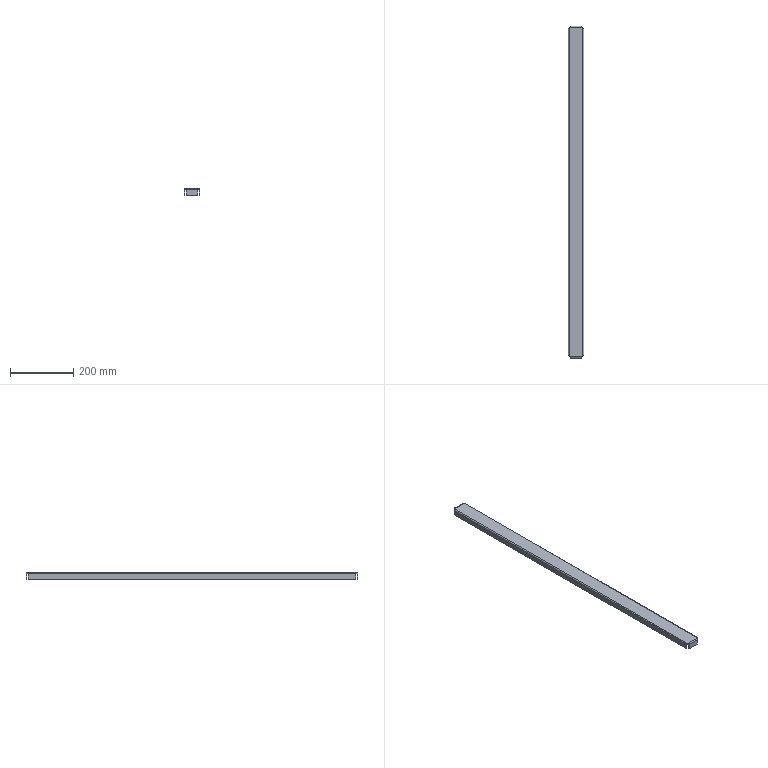Part | SolidWorks | features BaseBody 1 | 1 solid | 50 faces | box 50 x 1046 x 20 mm | volume 219402 mm3 | plane 42 | cylinder 8 | commonest cylinder face diameters 1.473 x4 6.473 x4
STEP:
#1=CARTESIAN_POINT('',(-18.,-520.5,-20.));
#2=VERTEX_POINT('',#1);
#3=CARTESIAN_POINT('',(18.,-520.5,-20.));
#4=VERTEX_POINT('',#3);
#5=CARTESIAN_POINT('',(18.,-520.5,-20.));
#6=DIRECTION('',(1.,0.,0.));
#7=VECTOR('',#6,1000.);
#8=LINE('',#5,#7);
#9=EDGE_CURVE('',#2,#4,#8,.T.);
#10=ORIENTED_EDGE('',*,*,#9,.T.);
#11=CARTESIAN_POINT('',(18.,-523.,-20.));
#12=VERTEX_POINT('',#11);
#13=CARTESIAN_POINT('',(18.,-523.,-20.));
#14=DIRECTION('',(0.,1.,0.));
#15=VECTOR('',#14,1000.);
#16=LINE('',#13,#15);
#17=EDGE_CURVE('',#12,#4,#16,.T.);
#18=ORIENTED_EDGE('',*,*,#17,.F.);
#19=CARTESIAN_POINT('',(-18.,-523.,-20.));
#20=VERTEX_POINT('',#19);
#21=CARTESIAN_POINT('',(0.,-523.,-20.));
#22=DIRECTION('',(1.,0.,0.));
#23=VECTOR('',#22,1000.);
#24=LINE('',#21,#23);
#25=EDGE_CURVE('',#20,#12,#24,.T.);
#26=ORIENTED_EDGE('',*,*,#25,.F.);
#27=CARTESIAN_POINT('',(-18.,-523.,-20.));
#28=DIRECTION('',(0.,1.,0.));
#29=VECTOR('',#28,1000.);
#30=LINE('',#27,#29);
#31=EDGE_CURVE('',#20,#2,#30,.T.);
#32=ORIENTED_EDGE('',*,*,#31,.T.);
#33=EDGE_LOOP('',(#10,#18,#26,#32));
#34=FACE_OUTER_BOUND('',#33,.T.);
#35=CARTESIAN_POINT('',(18.,-523.,-20.));
#36=DIRECTION('',(0.,0.,1.));
#37=DIRECTION('',(0.,-1.,0.));
#38=AXIS2_PLACEMENT_3D('',#35,#36,#37);
#39=PLANE('',#38);
#40=ADVANCED_FACE('',(#34),#39,.F.);
#41=CARTESIAN_POINT('',(-18.,-520.5,-3.237));
#42=VERTEX_POINT('',#41);
#43=CARTESIAN_POINT('',(-18.,-520.5,-20.));
#44=DIRECTION('',(0.,0.,-1.));
#45=VECTOR('',#44,1000.);
#46=LINE('',#43,#45);
#47=EDGE_CURVE('',#42,#2,#46,.T.);
#48=ORIENTED_EDGE('',*,*,#47,.F.);
#49=CARTESIAN_POINT('',(18.,-520.5,-3.237));
#50=VERTEX_POINT('',#49);
#51=CARTESIAN_POINT('',(18.,-520.5,-3.237));
#52=DIRECTION('',(-1.,0.,0.));
#53=VECTOR('',#52,1000.);
#54=LINE('',#51,#53);
#55=EDGE_CURVE('',#50,#42,#54,.T.);
#56=ORIENTED_EDGE('',*,*,#55,.F.);
#57=CARTESIAN_POINT('',(18.,-520.5,-2.5));
#58=DIRECTION('',(0.,0.,1.));
#59=VECTOR('',#58,1000.);
#60=LINE('',#57,#59);
#61=EDGE_CURVE('',#4,#50,#60,.T.);
#62=ORIENTED_EDGE('',*,*,#61,.F.);
#63=ORIENTED_EDGE('',*,*,#9,.F.);
#64=EDGE_LOOP('',(#48,#56,#62,#63));
#65=FACE_OUTER_BOUND('',#64,.T.);
#66=CARTESIAN_POINT('',(0.,-520.5,0.));
#67=DIRECTION('',(0.,1.,0.));
#68=DIRECTION('',(1.,0.,0.));
#69=AXIS2_PLACEMENT_3D('',#66,#67,#68);
#70=PLANE('',#69);
#71=ADVANCED_FACE('',(#65),#70,.T.);
#72=CARTESIAN_POINT('',(-18.,-523.,-3.237));
#73=VERTEX_POINT('',#72);
#74=CARTESIAN_POINT('',(18.,-523.,-3.237));
#75=VERTEX_POINT('',#74);
#76=CARTESIAN_POINT('',(18.,-523.,-3.237));
#77=DIRECTION('',(1.,0.,0.));
#78=VECTOR('',#77,1000.);
#79=LINE('',#76,#78);
#80=EDGE_CURVE('',#73,#75,#79,.T.);
#81=ORIENTED_EDGE('',*,*,#80,.F.);
#82=CARTESIAN_POINT('',(-18.,-523.,0.));
#83=DIRECTION('',(0.,0.,-1.));
#84=VECTOR('',#83,1000.);
#85=LINE('',#82,#84);
#86=EDGE_CURVE('',#73,#20,#85,.T.);
#87=ORIENTED_EDGE('',*,*,#86,.T.);
#88=ORIENTED_EDGE('',*,*,#25,.T.);
#89=CARTESIAN_POINT('',(18.,-523.,0.));
#90=DIRECTION('',(0.,0.,1.));
#91=VECTOR('',#90,1000.);
#92=LINE('',#89,#91);
#93=EDGE_CURVE('',#12,#75,#92,.T.);
#94=ORIENTED_EDGE('',*,*,#93,.T.);
#95=EDGE_LOOP('',(#81,#87,#88,#94));
#96=FACE_OUTER_BOUND('',#95,.T.);
#97=CARTESIAN_POINT('',(0.,-523.,0.));
#98=DIRECTION('',(0.,1.,0.));
#99=DIRECTION('',(1.,0.,0.));
#100=AXIS2_PLACEMENT_3D('',#97,#98,#99);
#101=PLANE('',#100);
#102=ADVANCED_FACE('',(#96),#101,.F.);
#103=CARTESIAN_POINT('',(18.,-523.,-3.237));
#104=DIRECTION('',(0.,-1.,0.));
#105=VECTOR('',#104,1000.);
#106=LINE('',#103,#105);
#107=EDGE_CURVE('',#50,#75,#106,.T.);
#108=ORIENTED_EDGE('',*,*,#107,.T.);
#109=ORIENTED_EDGE('',*,*,#93,.F.);
#110=ORIENTED_EDGE('',*,*,#17,.T.);
#111=ORIENTED_EDGE('',*,*,#61,.T.);
#112=EDGE_LOOP('',(#108,#109,#110,#111));
#113=FACE_OUTER_BOUND('',#112,.T.);
#114=CARTESIAN_POINT('',(18.,-523.,-2.5));
#115=DIRECTION('',(-1.,0.,0.));
#116=DIRECTION('',(0.,0.,1.));
#117=AXIS2_PLACEMENT_3D('',#114,#115,#116);
#118=PLANE('',#117);
#119=ADVANCED_FACE('',(#113),#118,.F.);
#120=CARTESIAN_POINT('',(-18.,-520.5,-3.237));
#121=DIRECTION('',(0.,-1.,0.));
#122=VECTOR('',#121,1000.);
#123=LINE('',#120,#122);
#124=EDGE_CURVE('',#42,#73,#123,.T.);
#125=ORIENTED_EDGE('',*,*,#124,.F.);
#126=ORIENTED_EDGE('',*,*,#47,.T.);
#127=ORIENTED_EDGE('',*,*,#31,.F.);
#128=ORIENTED_EDGE('',*,*,#86,.F.);
#129=EDGE_LOOP('',(#125,#126,#127,#128));
#130=FACE_OUTER_BOUND('',#129,.T.);
#131=CARTESIAN_POINT('',(-18.,-523.,-20.));
#132=DIRECTION('',(1.,0.,0.));
#133=DIRECTION('',(0.,-1.,0.));
#134=AXIS2_PLACEMENT_3D('',#131,#132,#133);
#135=PLANE('',#134);
#136=ADVANCED_FACE('',(#130),#135,.F.);
#137=CARTESIAN_POINT('',(-18.,-519.763,-2.5));
#138=VERTEX_POINT('',#137);
#139=CARTESIAN_POINT('',(18.,-519.763,-2.5));
#140=VERTEX_POINT('',#139);
#141=CARTESIAN_POINT('',(-18.,-519.763,-2.5));
#142=DIRECTION('',(1.,0.,0.));
#143=VECTOR('',#142,1000.);
#144=LINE('',#141,#143);
#145=EDGE_CURVE('',#138,#140,#144,.T.);
#146=ORIENTED_EDGE('',*,*,#145,.T.);
#147=CARTESIAN_POINT('',(18.,-519.763,-3.237));
#148=DIRECTION('',(1.,0.,0.));
#149=DIRECTION('',(0.,0.,1.));
#150=AXIS2_PLACEMENT_3D('',#147,#148,#149);
#151=CIRCLE('',#150,0.7366);
#152=EDGE_CURVE('',#140,#50,#151,.T.);
#153=ORIENTED_EDGE('',*,*,#152,.T.);
#154=ORIENTED_EDGE('',*,*,#55,.T.);
#155=CARTESIAN_POINT('',(-18.,-519.763,-3.237));
#156=DIRECTION('',(-1.,0.,0.));
#157=DIRECTION('',(0.,0.,1.));
#158=AXIS2_PLACEMENT_3D('',#155,#156,#157);
#159=CIRCLE('',#158,0.7366);
#160=EDGE_CURVE('',#42,#138,#159,.T.);
#161=ORIENTED_EDGE('',*,*,#160,.T.);
#162=EDGE_LOOP('',(#146,#153,#154,#161));
#163=FACE_OUTER_BOUND('',#162,.T.);
#164=CARTESIAN_POINT('',(-18.,-519.763,-3.237));
#165=DIRECTION('',(-1.,0.,0.));
#166=DIRECTION('',(0.,-1.,0.));
#167=AXIS2_PLACEMENT_3D('',#164,#165,#166);
#168=CYLINDRICAL_SURFACE('',#167,0.7366);
#169=ADVANCED_FACE('',(#163),#168,.F.);
#170=CARTESIAN_POINT('',(-18.,-519.763,0.));
#171=VERTEX_POINT('',#170);
#172=CARTESIAN_POINT('',(18.,-519.763,0.));
#173=VERTEX_POINT('',#172);
#174=CARTESIAN_POINT('',(-18.,-519.763,0.));
#175=DIRECTION('',(1.,0.,0.));
#176=VECTOR('',#175,1000.);
#177=LINE('',#174,#176);
#178=EDGE_CURVE('',#171,#173,#177,.T.);
#179=ORIENTED_EDGE('',*,*,#178,.F.);
#180=CARTESIAN_POINT('',(-18.,-522.915,-2.5));
#181=VERTEX_POINT('',#180);
#182=CARTESIAN_POINT('',(-18.,-519.763,-3.237));
#183=DIRECTION('',(-1.,0.,0.));
#184=DIRECTION('',(0.,0.,1.));
#185=AXIS2_PLACEMENT_3D('',#182,#183,#184);
#186=CIRCLE('',#185,3.237);
#187=EDGE_CURVE('',#181,#171,#186,.T.);
#188=ORIENTED_EDGE('',*,*,#187,.F.);
#189=CARTESIAN_POINT('',(-18.,-519.763,-3.237));
#190=DIRECTION('',(-1.,0.,0.));
#191=DIRECTION('',(0.,0.,1.));
#192=AXIS2_PLACEMENT_3D('',#189,#190,#191);
#193=CIRCLE('',#192,3.237);
#194=EDGE_CURVE('',#73,#181,#193,.T.);
#195=ORIENTED_EDGE('',*,*,#194,.F.);
#196=ORIENTED_EDGE('',*,*,#80,.T.);
#197=CARTESIAN_POINT('',(18.,-522.915,-2.5));
#198=VERTEX_POINT('',#197);
#199=CARTESIAN_POINT('',(18.,-519.763,-3.237));
#200=DIRECTION('',(1.,0.,0.));
#201=DIRECTION('',(0.,0.,1.));
#202=AXIS2_PLACEMENT_3D('',#199,#200,#201);
#203=CIRCLE('',#202,3.237);
#204=EDGE_CURVE('',#198,#75,#203,.T.);
#205=ORIENTED_EDGE('',*,*,#204,.F.);
#206=CARTESIAN_POINT('',(18.,-519.763,-3.237));
#207=DIRECTION('',(1.,0.,0.));
#208=DIRECTION('',(0.,0.,1.));
#209=AXIS2_PLACEMENT_3D('',#206,#207,#208);
#210=CIRCLE('',#209,3.237);
#211=EDGE_CURVE('',#173,#198,#210,.T.);
#212=ORIENTED_EDGE('',*,*,#211,.F.);
#213=EDGE_LOOP('',(#179,#188,#195,#196,#205,#212));
#214=FACE_OUTER_BOUND('',#213,.T.);
#215=CARTESIAN_POINT('',(-18.,-519.763,-3.237));
#216=DIRECTION('',(-1.,0.,0.));
#217=DIRECTION('',(0.,-1.,0.));
#218=AXIS2_PLACEMENT_3D('',#215,#216,#217);
#219=CYLINDRICAL_SURFACE('',#218,3.237);
#220=ADVANCED_FACE('',(#214),#219,.T.);
#221=ORIENTED_EDGE('',*,*,#194,.T.);
#222=CARTESIAN_POINT('',(-18.,-523.,-2.5));
#223=DIRECTION('',(0.,1.,0.));
#224=VECTOR('',#223,1000.);
#225=LINE('',#222,#224);
#226=EDGE_CURVE('',#181,#138,#225,.T.);
#227=ORIENTED_EDGE('',*,*,#226,.T.);
#228=ORIENTED_EDGE('',*,*,#160,.F.);
#229=ORIENTED_EDGE('',*,*,#124,.T.);
#230=EDGE_LOOP('',(#221,#227,#228,#229));
#231=FACE_OUTER_BOUND('',#230,.T.);
#232=CARTESIAN_POINT('',(-18.,-519.763,-3.237));
#233=DIRECTION('',(1.,0.,0.));
#234=DIRECTION('',(0.,1.,0.));
#235=AXIS2_PLACEMENT_3D('',#232,#233,#234);
#236=PLANE('',#235);
#237=ADVANCED_FACE('',(#231),#236,.F.);
#238=ORIENTED_EDGE('',*,*,#152,.F.);
#239=CARTESIAN_POINT('',(18.,-519.763,-2.5));
#240=DIRECTION('',(0.,-1.,0.));
#241=VECTOR('',#240,1000.);
#242=LINE('',#239,#241);
#243=EDGE_CURVE('',#140,#198,#242,.T.);
#244=ORIENTED_EDGE('',*,*,#243,.T.);
#245=ORIENTED_EDGE('',*,*,#204,.T.);
#246=ORIENTED_EDGE('',*,*,#107,.F.);
#247=EDGE_LOOP('',(#238,#244,#245,#246));
#248=FACE_OUTER_BOUND('',#247,.T.);
#249=CARTESIAN_POINT('',(18.,-519.763,-3.237));
#250=DIRECTION('',(1.,0.,0.));
#251=DIRECTION('',(0.,1.,0.));
#252=AXIS2_PLACEMENT_3D('',#249,#250,#251);
#253=PLANE('',#252);
#254=ADVANCED_FACE('',(#248),#253,.T.);
#255=CARTESIAN_POINT('',(22.5,-516.,-20.));
#256=VERTEX_POINT('',#255);
#257=CARTESIAN_POINT('',(22.5,516.,-20.));
#258=VERTEX_POINT('',#257);
#259=CARTESIAN_POINT('',(22.5,516.,-20.));
#260=DIRECTION('',(0.,1.,0.));
#261=VECTOR('',#260,1000.);
#262=LINE('',#259,#261);
#263=EDGE_CURVE('',#256,#258,#262,.T.);
#264=ORIENTED_EDGE('',*,*,#263,.T.);
#265=CARTESIAN_POINT('',(25.,516.,-20.));
#266=VERTEX_POINT('',#265);
#267=CARTESIAN_POINT('',(25.,516.,-20.));
#268=DIRECTION('',(-1.,0.,0.));
#269=VECTOR('',#268,1000.);
#270=LINE('',#267,#269);
#271=EDGE_CURVE('',#266,#258,#270,.T.);
#272=ORIENTED_EDGE('',*,*,#271,.F.);
#273=CARTESIAN_POINT('',(25.,-516.,-20.));
#274=VERTEX_POINT('',#273);
#275=CARTESIAN_POINT('',(25.,0.,-20.));
#276=DIRECTION('',(0.,1.,0.));
#277=VECTOR('',#276,1000.);
#278=LINE('',#275,#277);
#279=EDGE_CURVE('',#274,#266,#278,.T.);
#280=ORIENTED_EDGE('',*,*,#279,.F.);
#281=CARTESIAN_POINT('',(25.,-516.,-20.));
#282=DIRECTION('',(-1.,0.,0.));
#283=VECTOR('',#282,1000.);
#284=LINE('',#281,#283);
#285=EDGE_CURVE('',#274,#256,#284,.T.);
#286=ORIENTED_EDGE('',*,*,#285,.T.);
#287=EDGE_LOOP('',(#264,#272,#280,#286));
#288=FACE_OUTER_BOUND('',#287,.T.);
#289=CARTESIAN_POINT('',(25.,516.,-20.));
#290=DIRECTION('',(0.,0.,1.));
#291=DIRECTION('',(1.,0.,0.));
#292=AXIS2_PLACEMENT_3D('',#289,#290,#291);
#293=PLANE('',#292);
#294=ADVANCED_FACE('',(#288),#293,.F.);
#295=CARTESIAN_POINT('',(22.5,-516.,-3.237));
#296=VERTEX_POINT('',#295);
#297=CARTESIAN_POINT('',(22.5,-516.,-20.));
#298=DIRECTION('',(0.,0.,-1.));
#299=VECTOR('',#298,1000.);
#300=LINE('',#297,#299);
#301=EDGE_CURVE('',#296,#256,#300,.T.);
#302=ORIENTED_EDGE('',*,*,#301,.F.);
#303=CARTESIAN_POINT('',(22.5,516.,-3.237));
#304=VERTEX_POINT('',#303);
#305=CARTESIAN_POINT('',(22.5,516.,-3.237));
#306=DIRECTION('',(0.,-1.,0.));
#307=VECTOR('',#306,1000.);
#308=LINE('',#305,#307);
#309=EDGE_CURVE('',#304,#296,#308,.T.);
#310=ORIENTED_EDGE('',*,*,#309,.F.);
#311=CARTESIAN_POINT('',(22.5,516.,-2.5));
#312=DIRECTION('',(0.,0.,1.));
#313=VECTOR('',#312,1000.);
#314=LINE('',#311,#313);
#315=EDGE_CURVE('',#258,#304,#314,.T.);
#316=ORIENTED_EDGE('',*,*,#315,.F.);
#317=ORIENTED_EDGE('',*,*,#263,.F.);
#318=EDGE_LOOP('',(#302,#310,#316,#317));
#319=FACE_OUTER_BOUND('',#318,.T.);
#320=CARTESIAN_POINT('',(22.5,0.,0.));
#321=DIRECTION('',(-1.,0.,0.));
#322=DIRECTION('',(0.,0.,1.));
#323=AXIS2_PLACEMENT_3D('',#320,#321,#322);
#324=PLANE('',#323);
#325=ADVANCED_FACE('',(#319),#324,.T.);
#326=CARTESIAN_POINT('',(25.,-516.,-3.237));
#327=VERTEX_POINT('',#326);
#328=CARTESIAN_POINT('',(25.,516.,-3.237));
#329=VERTEX_POINT('',#328);
#330=CARTESIAN_POINT('',(25.,516.,-3.237));
#331=DIRECTION('',(0.,1.,0.));
#332=VECTOR('',#331,1000.);
#333=LINE('',#330,#332);
#334=EDGE_CURVE('',#327,#329,#333,.T.);
#335=ORIENTED_EDGE('',*,*,#334,.F.);
#336=CARTESIAN_POINT('',(25.,-516.,0.));
#337=DIRECTION('',(0.,0.,-1.));
#338=VECTOR('',#337,1000.);
#339=LINE('',#336,#338);
#340=EDGE_CURVE('',#327,#274,#339,.T.);
#341=ORIENTED_EDGE('',*,*,#340,.T.);
#342=ORIENTED_EDGE('',*,*,#279,.T.);
#343=CARTESIAN_POINT('',(25.,516.,0.));
#344=DIRECTION('',(0.,0.,1.));
#345=VECTOR('',#344,1000.);
#346=LINE('',#343,#345);
#347=EDGE_CURVE('',#266,#329,#346,.T.);
#348=ORIENTED_EDGE('',*,*,#347,.T.);
#349=EDGE_LOOP('',(#335,#341,#342,#348));
#350=FACE_OUTER_BOUND('',#349,.T.);
#351=CARTESIAN_POINT('',(25.,0.,0.));
#352=DIRECTION('',(-1.,0.,0.));
#353=DIRECTION('',(0.,0.,1.));
#354=AXIS2_PLACEMENT_3D('',#351,#352,#353);
#355=PLANE('',#354);
#356=ADVANCED_FACE('',(#350),#355,.F.);
#357=CARTESIAN_POINT('',(25.,516.,-3.237));
#358=DIRECTION('',(1.,0.,0.));
#359=VECTOR('',#358,1000.);
#360=LINE('',#357,#359);
#361=EDGE_CURVE('',#304,#329,#360,.T.);
#362=ORIENTED_EDGE('',*,*,#361,.T.);
#363=ORIENTED_EDGE('',*,*,#347,.F.);
#364=ORIENTED_EDGE('',*,*,#271,.T.);
#365=ORIENTED_EDGE('',*,*,#315,.T.);
#366=EDGE_LOOP('',(#362,#363,#364,#365));
#367=FACE_OUTER_BOUND('',#366,.T.);
#368=CARTESIAN_POINT('',(25.,516.,-2.5));
#369=DIRECTION('',(0.,-1.,0.));
#370=DIRECTION('',(-1.,0.,0.));
#371=AXIS2_PLACEMENT_3D('',#368,#369,#370);
#372=PLANE('',#371);
#373=ADVANCED_FACE('',(#367),#372,.F.);
#374=CARTESIAN_POINT('',(22.5,-516.,-3.237));
#375=DIRECTION('',(1.,0.,0.));
#376=VECTOR('',#375,1000.);
#377=LINE('',#374,#376);
#378=EDGE_CURVE('',#296,#327,#377,.T.);
#379=ORIENTED_EDGE('',*,*,#378,.F.);
#380=ORIENTED_EDGE('',*,*,#301,.T.);
#381=ORIENTED_EDGE('',*,*,#285,.F.);
#382=ORIENTED_EDGE('',*,*,#340,.F.);
#383=EDGE_LOOP('',(#379,#380,#381,#382));
#384=FACE_OUTER_BOUND('',#383,.T.);
#385=CARTESIAN_POINT('',(25.,-516.,-20.));
#386=DIRECTION('',(0.,1.,0.));
#387=DIRECTION('',(0.,0.,-1.));
#388=AXIS2_PLACEMENT_3D('',#385,#386,#387);
#389=PLANE('',#388);
#390=ADVANCED_FACE('',(#384),#389,.F.);
#391=CARTESIAN_POINT('',(21.763,-516.,-2.5));
#392=VERTEX_POINT('',#391);
#393=CARTESIAN_POINT('',(21.763,516.,-2.5));
#394=VERTEX_POINT('',#393);
#395=CARTESIAN_POINT('',(21.763,-516.,-2.5));
#396=DIRECTION('',(0.,1.,0.));
#397=VECTOR('',#396,1000.);
#398=LINE('',#395,#397);
#399=EDGE_CURVE('',#392,#394,#398,.T.);
#400=ORIENTED_EDGE('',*,*,#399,.T.);
#401=CARTESIAN_POINT('',(21.763,516.,-3.237));
#402=DIRECTION('',(0.,1.,0.));
#403=DIRECTION('',(0.,0.,-1.));
#404=AXIS2_PLACEMENT_3D('',#401,#402,#403);
#405=CIRCLE('',#404,0.7366);
#406=EDGE_CURVE('',#394,#304,#405,.T.);
#407=ORIENTED_EDGE('',*,*,#406,.T.);
#408=ORIENTED_EDGE('',*,*,#309,.T.);
#409=CARTESIAN_POINT('',(21.763,-516.,-3.237));
#410=DIRECTION('',(0.,-1.,0.));
#411=DIRECTION('',(0.,0.,-1.));
#412=AXIS2_PLACEMENT_3D('',#409,#410,#411);
#413=CIRCLE('',#412,0.7366);
#414=EDGE_CURVE('',#296,#392,#413,.T.);
#415=ORIENTED_EDGE('',*,*,#414,.T.);
#416=EDGE_LOOP('',(#400,#407,#408,#415));
#417=FACE_OUTER_BOUND('',#416,.T.);
#418=CARTESIAN_POINT('',(21.763,-516.,-3.237));
#419=DIRECTION('',(0.,-1.,0.));
#420=DIRECTION('',(1.,0.,0.));
#421=AXIS2_PLACEMENT_3D('',#418,#419,#420);
#422=CYLINDRICAL_SURFACE('',#421,0.7366);
#423=ADVANCED_FACE('',(#417),#422,.F.);
#424=CARTESIAN_POINT('',(21.763,-516.,0.));
#425=VERTEX_POINT('',#424);
#426=CARTESIAN_POINT('',(21.763,516.,0.));
#427=VERTEX_POINT('',#426);
#428=CARTESIAN_POINT('',(21.763,-516.,0.));
#429=DIRECTION('',(0.,1.,0.));
#430=VECTOR('',#429,1000.);
#431=LINE('',#428,#430);
#432=EDGE_CURVE('',#425,#427,#431,.T.);
#433=ORIENTED_EDGE('',*,*,#432,.F.);
#434=CARTESIAN_POINT('',(24.915,-516.,-2.5));
#435=VERTEX_POINT('',#434);
#436=CARTESIAN_POINT('',(21.763,-516.,-3.237));
#437=DIRECTION('',(0.,-1.,0.));
#438=DIRECTION('',(0.,0.,-1.));
#439=AXIS2_PLACEMENT_3D('',#436,#437,#438);
#440=CIRCLE('',#439,3.237);
#441=EDGE_CURVE('',#435,#425,#440,.T.);
#442=ORIENTED_EDGE('',*,*,#441,.F.);
#443=CARTESIAN_POINT('',(21.763,-516.,-3.237));
#444=DIRECTION('',(0.,-1.,0.));
#445=DIRECTION('',(0.,0.,-1.));
#446=AXIS2_PLACEMENT_3D('',#443,#444,#445);
#447=CIRCLE('',#446,3.237);
#448=EDGE_CURVE('',#327,#435,#447,.T.);
#449=ORIENTED_EDGE('',*,*,#448,.F.);
#450=ORIENTED_EDGE('',*,*,#334,.T.);
#451=CARTESIAN_POINT('',(24.915,516.,-2.5));
#452=VERTEX_POINT('',#451);
#453=CARTESIAN_POINT('',(21.763,516.,-3.237));
#454=DIRECTION('',(0.,1.,0.));
#455=DIRECTION('',(0.,0.,-1.));
#456=AXIS2_PLACEMENT_3D('',#453,#454,#455);
#457=CIRCLE('',#456,3.237);
#458=EDGE_CURVE('',#452,#329,#457,.T.);
#459=ORIENTED_EDGE('',*,*,#458,.F.);
#460=CARTESIAN_POINT('',(21.763,516.,-3.237));
#461=DIRECTION('',(0.,1.,0.));
#462=DIRECTION('',(0.,0.,-1.));
#463=AXIS2_PLACEMENT_3D('',#460,#461,#462);
#464=CIRCLE('',#463,3.237);
#465=EDGE_CURVE('',#427,#452,#464,.T.);
#466=ORIENTED_EDGE('',*,*,#465,.F.);
#467=EDGE_LOOP('',(#433,#442,#449,#450,#459,#466));
#468=FACE_OUTER_BOUND('',#467,.T.);
#469=CARTESIAN_POINT('',(21.763,-516.,-3.237));
#470=DIRECTION('',(0.,-1.,0.));
#471=DIRECTION('',(1.,0.,0.));
#472=AXIS2_PLACEMENT_3D('',#469,#470,#471);
#473=CYLINDRICAL_SURFACE('',#472,3.237);
#474=ADVANCED_FACE('',(#468),#473,.T.);
#475=ORIENTED_EDGE('',*,*,#448,.T.);
#476=CARTESIAN_POINT('',(25.,-516.,-2.5));
#477=DIRECTION('',(-1.,0.,0.));
#478=VECTOR('',#477,1000.);
#479=LINE('',#476,#478);
#480=EDGE_CURVE('',#435,#392,#479,.T.);
#481=ORIENTED_EDGE('',*,*,#480,.T.);
#482=ORIENTED_EDGE('',*,*,#414,.F.);
#483=ORIENTED_EDGE('',*,*,#378,.T.);
#484=EDGE_LOOP('',(#475,#481,#482,#483));
#485=FACE_OUTER_BOUND('',#484,.T.);
#486=CARTESIAN_POINT('',(21.763,-516.,-3.237));
#487=DIRECTION('',(0.,1.,0.));
#488=DIRECTION('',(1.,0.,0.));
#489=AXIS2_PLACEMENT_3D('',#486,#487,#488);
#490=PLANE('',#489);
#491=ADVANCED_FACE('',(#485),#490,.F.);
#492=ORIENTED_EDGE('',*,*,#406,.F.);
#493=CARTESIAN_POINT('',(21.763,516.,-2.5));
#494=DIRECTION('',(1.,0.,0.));
#495=VECTOR('',#494,1000.);
#496=LINE('',#493,#495);
#497=EDGE_CURVE('',#394,#452,#496,.T.);
#498=ORIENTED_EDGE('',*,*,#497,.T.);
#499=ORIENTED_EDGE('',*,*,#458,.T.);
#500=ORIENTED_EDGE('',*,*,#361,.F.);
#501=EDGE_LOOP('',(#492,#498,#499,#500));
#502=FACE_OUTER_BOUND('',#501,.T.);
#503=CARTESIAN_POINT('',(21.763,516.,-3.237));
#504=DIRECTION('',(0.,1.,0.));
#505=DIRECTION('',(1.,0.,0.));
#506=AXIS2_PLACEMENT_3D('',#503,#504,#505);
#507=PLANE('',#506);
#508=ADVANCED_FACE('',(#502),#507,.T.);
#509=CARTESIAN_POINT('',(18.,520.5,-20.));
#510=VERTEX_POINT('',#509);
#511=CARTESIAN_POINT('',(-18.,520.5,-20.));
#512=VERTEX_POINT('',#511);
#513=CARTESIAN_POINT('',(-18.,520.5,-20.));
#514=DIRECTION('',(-1.,0.,0.));
#515=VECTOR('',#514,1000.);
#516=LINE('',#513,#515);
#517=EDGE_CURVE('',#510,#512,#516,.T.);
#518=ORIENTED_EDGE('',*,*,#517,.T.);
#519=CARTESIAN_POINT('',(-18.,523.,-20.));
#520=VERTEX_POINT('',#519);
#521=CARTESIAN_POINT('',(-18.,523.,-20.));
#522=DIRECTION('',(0.,-1.,0.));
#523=VECTOR('',#522,1000.);
#524=LINE('',#521,#523);
#525=EDGE_CURVE('',#520,#512,#524,.T.);
#526=ORIENTED_EDGE('',*,*,#525,.F.);
#527=CARTESIAN_POINT('',(18.,523.,-20.));
#528=VERTEX_POINT('',#527);
#529=CARTESIAN_POINT('',(0.,523.,-20.));
#530=DIRECTION('',(-1.,0.,0.));
#531=VECTOR('',#530,1000.);
#532=LINE('',#529,#531);
#533=EDGE_CURVE('',#528,#520,#532,.T.);
#534=ORIENTED_EDGE('',*,*,#533,.F.);
#535=CARTESIAN_POINT('',(18.,523.,-20.));
#536=DIRECTION('',(0.,-1.,0.));
#537=VECTOR('',#536,1000.);
#538=LINE('',#535,#537);
#539=EDGE_CURVE('',#528,#510,#538,.T.);
#540=ORIENTED_EDGE('',*,*,#539,.T.);
#541=EDGE_LOOP('',(#518,#526,#534,#540));
#542=FACE_OUTER_BOUND('',#541,.T.);
#543=CARTESIAN_POINT('',(-18.,523.,-20.));
#544=DIRECTION('',(0.,0.,1.));
#545=DIRECTION('',(0.,-1.,0.));
#546=AXIS2_PLACEMENT_3D('',#543,#544,#545);
#547=PLANE('',#546);
#548=ADVANCED_FACE('',(#542),#547,.F.);
#549=CARTESIAN_POINT('',(18.,520.5,-3.237));
#550=VERTEX_POINT('',#549);
#551=CARTESIAN_POINT('',(18.,520.5,-20.));
#552=DIRECTION('',(0.,0.,-1.));
#553=VECTOR('',#552,1000.);
#554=LINE('',#551,#553);
#555=EDGE_CURVE('',#550,#510,#554,.T.);
#556=ORIENTED_EDGE('',*,*,#555,.F.);
#557=CARTESIAN_POINT('',(-18.,520.5,-3.237));
#558=VERTEX_POINT('',#557);
#559=CARTESIAN_POINT('',(-18.,520.5,-3.237));
#560=DIRECTION('',(1.,0.,0.));
#561=VECTOR('',#560,1000.);
#562=LINE('',#559,#561);
#563=EDGE_CURVE('',#558,#550,#562,.T.);
#564=ORIENTED_EDGE('',*,*,#563,.F.);
#565=CARTESIAN_POINT('',(-18.,520.5,-2.5));
#566=DIRECTION('',(0.,0.,1.));
#567=VECTOR('',#566,1000.);
#568=LINE('',#565,#567);
#569=EDGE_CURVE('',#512,#558,#568,.T.);
#570=ORIENTED_EDGE('',*,*,#569,.F.);
#571=ORIENTED_EDGE('',*,*,#517,.F.);
#572=EDGE_LOOP('',(#556,#564,#570,#571));
#573=FACE_OUTER_BOUND('',#572,.T.);
#574=CARTESIAN_POINT('',(0.,520.5,0.));
#575=DIRECTION('',(0.,-1.,0.));
#576=DIRECTION('',(0.,0.,-1.));
#577=AXIS2_PLACEMENT_3D('',#574,#575,#576);
#578=PLANE('',#577);
#579=ADVANCED_FACE('',(#573),#578,.T.);
#580=CARTESIAN_POINT('',(18.,523.,-3.237));
#581=VERTEX_POINT('',#580);
#582=CARTESIAN_POINT('',(-18.,523.,-3.237));
#583=VERTEX_POINT('',#582);
#584=CARTESIAN_POINT('',(-18.,523.,-3.237));
#585=DIRECTION('',(-1.,0.,0.));
#586=VECTOR('',#585,1000.);
#587=LINE('',#584,#586);
#588=EDGE_CURVE('',#581,#583,#587,.T.);
#589=ORIENTED_EDGE('',*,*,#588,.F.);
#590=CARTESIAN_POINT('',(18.,523.,0.));
#591=DIRECTION('',(0.,0.,-1.));
#592=VECTOR('',#591,1000.);
#593=LINE('',#590,#592);
#594=EDGE_CURVE('',#581,#528,#593,.T.);
#595=ORIENTED_EDGE('',*,*,#594,.T.);
#596=ORIENTED_EDGE('',*,*,#533,.T.);
#597=CARTESIAN_POINT('',(-18.,523.,0.));
#598=DIRECTION('',(0.,0.,1.));
#599=VECTOR('',#598,1000.);
#600=LINE('',#597,#599);
#601=EDGE_CURVE('',#520,#583,#600,.T.);
#602=ORIENTED_EDGE('',*,*,#601,.T.);
#603=EDGE_LOOP('',(#589,#595,#596,#602));
#604=FACE_OUTER_BOUND('',#603,.T.);
#605=CARTESIAN_POINT('',(0.,523.,0.));
#606=DIRECTION('',(0.,-1.,0.));
#607=DIRECTION('',(0.,0.,-1.));
#608=AXIS2_PLACEMENT_3D('',#605,#606,#607);
#609=PLANE('',#608);
#610=ADVANCED_FACE('',(#604),#609,.F.);
#611=CARTESIAN_POINT('',(-18.,523.,-3.237));
#612=DIRECTION('',(0.,1.,0.));
#613=VECTOR('',#612,1000.);
#614=LINE('',#611,#613);
#615=EDGE_CURVE('',#558,#583,#614,.T.);
#616=ORIENTED_EDGE('',*,*,#615,.T.);
#617=ORIENTED_EDGE('',*,*,#601,.F.);
#618=ORIENTED_EDGE('',*,*,#525,.T.);
#619=ORIENTED_EDGE('',*,*,#569,.T.);
#620=EDGE_LOOP('',(#616,#617,#618,#619));
#621=FACE_OUTER_BOUND('',#620,.T.);
#622=CARTESIAN_POINT('',(-18.,523.,-2.5));
#623=DIRECTION('',(1.,0.,0.));
#624=DIRECTION('',(0.,1.,0.));
#625=AXIS2_PLACEMENT_3D('',#622,#623,#624);
#626=PLANE('',#625);
#627=ADVANCED_FACE('',(#621),#626,.F.);
#628=CARTESIAN_POINT('',(18.,520.5,-3.237));
#629=DIRECTION('',(0.,1.,0.));
#630=VECTOR('',#629,1000.);
#631=LINE('',#628,#630);
#632=EDGE_CURVE('',#550,#581,#631,.T.);
#633=ORIENTED_EDGE('',*,*,#632,.F.);
#634=ORIENTED_EDGE('',*,*,#555,.T.);
#635=ORIENTED_EDGE('',*,*,#539,.F.);
#636=ORIENTED_EDGE('',*,*,#594,.F.);
#637=EDGE_LOOP('',(#633,#634,#635,#636));
#638=FACE_OUTER_BOUND('',#637,.T.);
#639=CARTESIAN_POINT('',(18.,523.,-20.));
#640=DIRECTION('',(-1.,0.,0.));
#641=DIRECTION('',(0.,1.,0.));
#642=AXIS2_PLACEMENT_3D('',#639,#640,#641);
#643=PLANE('',#642);
#644=ADVANCED_FACE('',(#638),#643,.F.);
#645=CARTESIAN_POINT('',(18.,519.763,-2.5));
#646=VERTEX_POINT('',#645);
#647=CARTESIAN_POINT('',(-18.,519.763,-2.5));
#648=VERTEX_POINT('',#647);
#649=CARTESIAN_POINT('',(18.,519.763,-2.5));
#650=DIRECTION('',(-1.,0.,0.));
#651=VECTOR('',#650,1000.);
#652=LINE('',#649,#651);
#653=EDGE_CURVE('',#646,#648,#652,.T.);
#654=ORIENTED_EDGE('',*,*,#653,.T.);
#655=CARTESIAN_POINT('',(-18.,519.763,-3.237));
#656=DIRECTION('',(-1.,0.,0.));
#657=DIRECTION('',(0.,0.,-1.));
#658=AXIS2_PLACEMENT_3D('',#655,#656,#657);
#659=CIRCLE('',#658,0.7366);
#660=EDGE_CURVE('',#648,#558,#659,.T.);
#661=ORIENTED_EDGE('',*,*,#660,.T.);
#662=ORIENTED_EDGE('',*,*,#563,.T.);
#663=CARTESIAN_POINT('',(18.,519.763,-3.237));
#664=DIRECTION('',(1.,0.,0.));
#665=DIRECTION('',(0.,0.,-1.));
#666=AXIS2_PLACEMENT_3D('',#663,#664,#665);
#667=CIRCLE('',#666,0.7366);
#668=EDGE_CURVE('',#550,#646,#667,.T.);
#669=ORIENTED_EDGE('',*,*,#668,.T.);
#670=EDGE_LOOP('',(#654,#661,#662,#669));
#671=FACE_OUTER_BOUND('',#670,.T.);
#672=CARTESIAN_POINT('',(18.,519.763,-3.237));
#673=DIRECTION('',(1.,0.,0.));
#674=DIRECTION('',(0.,1.,0.));
#675=AXIS2_PLACEMENT_3D('',#672,#673,#674);
#676=CYLINDRICAL_SURFACE('',#675,0.7366);
#677=ADVANCED_FACE('',(#671),#676,.F.);
#678=CARTESIAN_POINT('',(18.,519.763,0.));
#679=VERTEX_POINT('',#678);
#680=CARTESIAN_POINT('',(-18.,519.763,0.));
#681=VERTEX_POINT('',#680);
#682=CARTESIAN_POINT('',(18.,519.763,0.));
#683=DIRECTION('',(-1.,0.,0.));
#684=VECTOR('',#683,1000.);
#685=LINE('',#682,#684);
#686=EDGE_CURVE('',#679,#681,#685,.T.);
#687=ORIENTED_EDGE('',*,*,#686,.F.);
#688=CARTESIAN_POINT('',(18.,522.915,-2.5));
#689=VERTEX_POINT('',#688);
#690=CARTESIAN_POINT('',(18.,519.763,-3.237));
#691=DIRECTION('',(1.,0.,0.));
#692=DIRECTION('',(0.,0.,-1.));
#693=AXIS2_PLACEMENT_3D('',#690,#691,#692);
#694=CIRCLE('',#693,3.237);
#695=EDGE_CURVE('',#689,#679,#694,.T.);
#696=ORIENTED_EDGE('',*,*,#695,.F.);
#697=CARTESIAN_POINT('',(18.,519.763,-3.237));
#698=DIRECTION('',(1.,0.,0.));
#699=DIRECTION('',(0.,0.,-1.));
#700=AXIS2_PLACEMENT_3D('',#697,#698,#699);
#701=CIRCLE('',#700,3.237);
#702=EDGE_CURVE('',#581,#689,#701,.T.);
#703=ORIENTED_EDGE('',*,*,#702,.F.);
#704=ORIENTED_EDGE('',*,*,#588,.T.);
#705=CARTESIAN_POINT('',(-18.,522.915,-2.5));
#706=VERTEX_POINT('',#705);
#707=CARTESIAN_POINT('',(-18.,519.763,-3.237));
#708=DIRECTION('',(-1.,0.,0.));
#709=DIRECTION('',(0.,0.,-1.));
#710=AXIS2_PLACEMENT_3D('',#707,#708,#709);
#711=CIRCLE('',#710,3.237);
#712=EDGE_CURVE('',#706,#583,#711,.T.);
#713=ORIENTED_EDGE('',*,*,#712,.F.);
#714=CARTESIAN_POINT('',(-18.,519.763,-3.237));
#715=DIRECTION('',(-1.,0.,0.));
#716=DIRECTION('',(0.,0.,-1.));
#717=AXIS2_PLACEMENT_3D('',#714,#715,#716);
#718=CIRCLE('',#717,3.237);
#719=EDGE_CURVE('',#681,#706,#718,.T.);
#720=ORIENTED_EDGE('',*,*,#719,.F.);
#721=EDGE_LOOP('',(#687,#696,#703,#704,#713,#720));
#722=FACE_OUTER_BOUND('',#721,.T.);
#723=CARTESIAN_POINT('',(18.,519.763,-3.237));
#724=DIRECTION('',(1.,0.,0.));
#725=DIRECTION('',(0.,1.,0.));
#726=AXIS2_PLACEMENT_3D('',#723,#724,#725);
#727=CYLINDRICAL_SURFACE('',#726,3.237);
#728=ADVANCED_FACE('',(#722),#727,.T.);
#729=ORIENTED_EDGE('',*,*,#702,.T.);
#730=CARTESIAN_POINT('',(18.,523.,-2.5));
#731=DIRECTION('',(0.,-1.,0.));
#732=VECTOR('',#731,1000.);
#733=LINE('',#730,#732);
#734=EDGE_CURVE('',#689,#646,#733,.T.);
#735=ORIENTED_EDGE('',*,*,#734,.T.);
#736=ORIENTED_EDGE('',*,*,#668,.F.);
#737=ORIENTED_EDGE('',*,*,#632,.T.);
#738=EDGE_LOOP('',(#729,#735,#736,#737));
#739=FACE_OUTER_BOUND('',#738,.T.);
#740=CARTESIAN_POINT('',(18.,519.763,-3.237));
#741=DIRECTION('',(-1.,0.,0.));
#742=DIRECTION('',(0.,0.,1.));
#743=AXIS2_PLACEMENT_3D('',#740,#741,#742);
#744=PLANE('',#743);
#745=ADVANCED_FACE('',(#739),#744,.F.);
#746=ORIENTED_EDGE('',*,*,#660,.F.);
#747=CARTESIAN_POINT('',(-18.,519.763,-2.5));
#748=DIRECTION('',(0.,1.,0.));
#749=VECTOR('',#748,1000.);
#750=LINE('',#747,#749);
#751=EDGE_CURVE('',#648,#706,#750,.T.);
#752=ORIENTED_EDGE('',*,*,#751,.T.);
#753=ORIENTED_EDGE('',*,*,#712,.T.);
#754=ORIENTED_EDGE('',*,*,#615,.F.);
#755=EDGE_LOOP('',(#746,#752,#753,#754));
#756=FACE_OUTER_BOUND('',#755,.T.);
#757=CARTESIAN_POINT('',(-18.,519.763,-3.237));
#758=DIRECTION('',(-1.,0.,0.));
#759=DIRECTION('',(0.,0.,1.));
#760=AXIS2_PLACEMENT_3D('',#757,#758,#759);
#761=PLANE('',#760);
#762=ADVANCED_FACE('',(#756),#761,.T.);
#763=CARTESIAN_POINT('',(-22.5,516.,-20.));
#764=VERTEX_POINT('',#763);
#765=CARTESIAN_POINT('',(-22.5,-516.,-20.));
#766=VERTEX_POINT('',#765);
#767=CARTESIAN_POINT('',(-22.5,-516.,-20.));
#768=DIRECTION('',(0.,-1.,0.));
#769=VECTOR('',#768,1000.);
#770=LINE('',#767,#769);
#771=EDGE_CURVE('',#764,#766,#770,.T.);
#772=ORIENTED_EDGE('',*,*,#771,.T.);
#773=CARTESIAN_POINT('',(-25.,-516.,-20.));
#774=VERTEX_POINT('',#773);
#775=CARTESIAN_POINT('',(-25.,-516.,-20.));
#776=DIRECTION('',(1.,0.,0.));
#777=VECTOR('',#776,1000.);
#778=LINE('',#775,#777);
#779=EDGE_CURVE('',#774,#766,#778,.T.);
#780=ORIENTED_EDGE('',*,*,#779,.F.);
#781=CARTESIAN_POINT('',(-25.,516.,-20.));
#782=VERTEX_POINT('',#781);
#783=CARTESIAN_POINT('',(-25.,0.,-20.));
#784=DIRECTION('',(0.,-1.,0.));
#785=VECTOR('',#784,1000.);
#786=LINE('',#783,#785);
#787=EDGE_CURVE('',#782,#774,#786,.T.);
#788=ORIENTED_EDGE('',*,*,#787,.F.);
#789=CARTESIAN_POINT('',(-25.,516.,-20.));
#790=DIRECTION('',(1.,0.,0.));
#791=VECTOR('',#790,1000.);
#792=LINE('',#789,#791);
#793=EDGE_CURVE('',#782,#764,#792,.T.);
#794=ORIENTED_EDGE('',*,*,#793,.T.);
#795=EDGE_LOOP('',(#772,#780,#788,#794));
#796=FACE_OUTER_BOUND('',#795,.T.);
#797=CARTESIAN_POINT('',(-25.,-516.,-20.));
#798=DIRECTION('',(0.,0.,1.));
#799=DIRECTION('',(1.,0.,0.));
#800=AXIS2_PLACEMENT_3D('',#797,#798,#799);
#801=PLANE('',#800);
#802=ADVANCED_FACE('',(#796),#801,.F.);
#803=CARTESIAN_POINT('',(-22.5,516.,-3.237));
#804=VERTEX_POINT('',#803);
#805=CARTESIAN_POINT('',(-22.5,516.,-20.));
#806=DIRECTION('',(0.,0.,-1.));
#807=VECTOR('',#806,1000.);
#808=LINE('',#805,#807);
#809=EDGE_CURVE('',#804,#764,#808,.T.);
#810=ORIENTED_EDGE('',*,*,#809,.F.);
#811=CARTESIAN_POINT('',(-22.5,-516.,-3.237));
#812=VERTEX_POINT('',#811);
#813=CARTESIAN_POINT('',(-22.5,-516.,-3.237));
#814=DIRECTION('',(0.,1.,0.));
#815=VECTOR('',#814,1000.);
#816=LINE('',#813,#815);
#817=EDGE_CURVE('',#812,#804,#816,.T.);
#818=ORIENTED_EDGE('',*,*,#817,.F.);
#819=CARTESIAN_POINT('',(-22.5,-516.,-2.5));
#820=DIRECTION('',(0.,0.,1.));
#821=VECTOR('',#820,1000.);
#822=LINE('',#819,#821);
#823=EDGE_CURVE('',#766,#812,#822,.T.);
#824=ORIENTED_EDGE('',*,*,#823,.F.);
#825=ORIENTED_EDGE('',*,*,#771,.F.);
#826=EDGE_LOOP('',(#810,#818,#824,#825));
#827=FACE_OUTER_BOUND('',#826,.T.);
#828=CARTESIAN_POINT('',(-22.5,0.,0.));
#829=DIRECTION('',(1.,0.,0.));
#830=DIRECTION('',(0.,0.,-1.));
#831=AXIS2_PLACEMENT_3D('',#828,#829,#830);
#832=PLANE('',#831);
#833=ADVANCED_FACE('',(#827),#832,.T.);
#834=CARTESIAN_POINT('',(-25.,516.,-3.237));
#835=VERTEX_POINT('',#834);
#836=CARTESIAN_POINT('',(-25.,-516.,-3.237));
#837=VERTEX_POINT('',#836);
#838=CARTESIAN_POINT('',(-25.,-516.,-3.237));
#839=DIRECTION('',(0.,-1.,0.));
#840=VECTOR('',#839,1000.);
#841=LINE('',#838,#840);
#842=EDGE_CURVE('',#835,#837,#841,.T.);
#843=ORIENTED_EDGE('',*,*,#842,.F.);
#844=CARTESIAN_POINT('',(-25.,516.,0.));
#845=DIRECTION('',(0.,0.,-1.));
#846=VECTOR('',#845,1000.);
#847=LINE('',#844,#846);
#848=EDGE_CURVE('',#835,#782,#847,.T.);
#849=ORIENTED_EDGE('',*,*,#848,.T.);
#850=ORIENTED_EDGE('',*,*,#787,.T.);
#851=CARTESIAN_POINT('',(-25.,-516.,0.));
#852=DIRECTION('',(0.,0.,1.));
#853=VECTOR('',#852,1000.);
#854=LINE('',#851,#853);
#855=EDGE_CURVE('',#774,#837,#854,.T.);
#856=ORIENTED_EDGE('',*,*,#855,.T.);
#857=EDGE_LOOP('',(#843,#849,#850,#856));
#858=FACE_OUTER_BOUND('',#857,.T.);
#859=CARTESIAN_POINT('',(-25.,0.,0.));
#860=DIRECTION('',(1.,0.,0.));
#861=DIRECTION('',(0.,0.,-1.));
#862=AXIS2_PLACEMENT_3D('',#859,#860,#861);
#863=PLANE('',#862);
#864=ADVANCED_FACE('',(#858),#863,.F.);
#865=CARTESIAN_POINT('',(-25.,-516.,-3.237));
#866=DIRECTION('',(-1.,0.,0.));
#867=VECTOR('',#866,1000.);
#868=LINE('',#865,#867);
#869=EDGE_CURVE('',#812,#837,#868,.T.);
#870=ORIENTED_EDGE('',*,*,#869,.T.);
#871=ORIENTED_EDGE('',*,*,#855,.F.);
#872=ORIENTED_EDGE('',*,*,#779,.T.);
#873=ORIENTED_EDGE('',*,*,#823,.T.);
#874=EDGE_LOOP('',(#870,#871,#872,#873));
#875=FACE_OUTER_BOUND('',#874,.T.);
#876=CARTESIAN_POINT('',(-25.,-516.,-2.5));
#877=DIRECTION('',(0.,1.,0.));
#878=DIRECTION('',(0.,0.,-1.));
#879=AXIS2_PLACEMENT_3D('',#876,#877,#878);
#880=PLANE('',#879);
#881=ADVANCED_FACE('',(#875),#880,.F.);
#882=CARTESIAN_POINT('',(-22.5,516.,-3.237));
#883=DIRECTION('',(-1.,0.,0.));
#884=VECTOR('',#883,1000.);
#885=LINE('',#882,#884);
#886=EDGE_CURVE('',#804,#835,#885,.T.);
#887=ORIENTED_EDGE('',*,*,#886,.F.);
#888=ORIENTED_EDGE('',*,*,#809,.T.);
#889=ORIENTED_EDGE('',*,*,#793,.F.);
#890=ORIENTED_EDGE('',*,*,#848,.F.);
#891=EDGE_LOOP('',(#887,#888,#889,#890));
#892=FACE_OUTER_BOUND('',#891,.T.);
#893=CARTESIAN_POINT('',(-25.,516.,-20.));
#894=DIRECTION('',(0.,-1.,0.));
#895=DIRECTION('',(-1.,0.,0.));
#896=AXIS2_PLACEMENT_3D('',#893,#894,#895);
#897=PLANE('',#896);
#898=ADVANCED_FACE('',(#892),#897,.F.);
#899=CARTESIAN_POINT('',(-21.763,516.,-2.5));
#900=VERTEX_POINT('',#899);
#901=CARTESIAN_POINT('',(-21.763,-516.,-2.5));
#902=VERTEX_POINT('',#901);
#903=CARTESIAN_POINT('',(-21.763,516.,-2.5));
#904=DIRECTION('',(0.,-1.,0.));
#905=VECTOR('',#904,1000.);
#906=LINE('',#903,#905);
#907=EDGE_CURVE('',#900,#902,#906,.T.);
#908=ORIENTED_EDGE('',*,*,#907,.T.);
#909=CARTESIAN_POINT('',(-21.763,-516.,-3.237));
#910=DIRECTION('',(0.,-1.,0.));
#911=DIRECTION('',(0.,0.,1.));
#912=AXIS2_PLACEMENT_3D('',#909,#910,#911);
#913=CIRCLE('',#912,0.7366);
#914=EDGE_CURVE('',#902,#812,#913,.T.);
#915=ORIENTED_EDGE('',*,*,#914,.T.);
#916=ORIENTED_EDGE('',*,*,#817,.T.);
#917=CARTESIAN_POINT('',(-21.763,516.,-3.237));
#918=DIRECTION('',(0.,1.,0.));
#919=DIRECTION('',(0.,0.,1.));
#920=AXIS2_PLACEMENT_3D('',#917,#918,#919);
#921=CIRCLE('',#920,0.7366);
#922=EDGE_CURVE('',#804,#900,#921,.T.);
#923=ORIENTED_EDGE('',*,*,#922,.T.);
#924=EDGE_LOOP('',(#908,#915,#916,#923));
#925=FACE_OUTER_BOUND('',#924,.T.);
#926=CARTESIAN_POINT('',(-21.763,516.,-3.237));
#927=DIRECTION('',(0.,1.,0.));
#928=DIRECTION('',(-1.,0.,0.));
#929=AXIS2_PLACEMENT_3D('',#926,#927,#928);
#930=CYLINDRICAL_SURFACE('',#929,0.7366);
#931=ADVANCED_FACE('',(#925),#930,.F.);
#932=CARTESIAN_POINT('',(-21.763,516.,0.));
#933=VERTEX_POINT('',#932);
#934=CARTESIAN_POINT('',(-21.763,-516.,0.));
#935=VERTEX_POINT('',#934);
#936=CARTESIAN_POINT('',(-21.763,516.,0.));
#937=DIRECTION('',(0.,-1.,0.));
#938=VECTOR('',#937,1000.);
#939=LINE('',#936,#938);
#940=EDGE_CURVE('',#933,#935,#939,.T.);
#941=ORIENTED_EDGE('',*,*,#940,.F.);
#942=CARTESIAN_POINT('',(-24.915,516.,-2.5));
#943=VERTEX_POINT('',#942);
#944=CARTESIAN_POINT('',(-21.763,516.,-3.237));
#945=DIRECTION('',(0.,1.,0.));
#946=DIRECTION('',(0.,0.,1.));
#947=AXIS2_PLACEMENT_3D('',#944,#945,#946);
#948=CIRCLE('',#947,3.237);
#949=EDGE_CURVE('',#943,#933,#948,.T.);
#950=ORIENTED_EDGE('',*,*,#949,.F.);
#951=CARTESIAN_POINT('',(-21.763,516.,-3.237));
#952=DIRECTION('',(0.,1.,0.));
#953=DIRECTION('',(0.,0.,1.));
#954=AXIS2_PLACEMENT_3D('',#951,#952,#953);
#955=CIRCLE('',#954,3.237);
#956=EDGE_CURVE('',#835,#943,#955,.T.);
#957=ORIENTED_EDGE('',*,*,#956,.F.);
#958=ORIENTED_EDGE('',*,*,#842,.T.);
#959=CARTESIAN_POINT('',(-24.915,-516.,-2.5));
#960=VERTEX_POINT('',#959);
#961=CARTESIAN_POINT('',(-21.763,-516.,-3.237));
#962=DIRECTION('',(0.,-1.,0.));
#963=DIRECTION('',(0.,0.,1.));
#964=AXIS2_PLACEMENT_3D('',#961,#962,#963);
#965=CIRCLE('',#964,3.237);
#966=EDGE_CURVE('',#960,#837,#965,.T.);
#967=ORIENTED_EDGE('',*,*,#966,.F.);
#968=CARTESIAN_POINT('',(-21.763,-516.,-3.237));
#969=DIRECTION('',(0.,-1.,0.));
#970=DIRECTION('',(0.,0.,1.));
#971=AXIS2_PLACEMENT_3D('',#968,#969,#970);
#972=CIRCLE('',#971,3.237);
#973=EDGE_CURVE('',#935,#960,#972,.T.);
#974=ORIENTED_EDGE('',*,*,#973,.F.);
#975=EDGE_LOOP('',(#941,#950,#957,#958,#967,#974));
#976=FACE_OUTER_BOUND('',#975,.T.);
#977=CARTESIAN_POINT('',(-21.763,516.,-3.237));
#978=DIRECTION('',(0.,1.,0.));
#979=DIRECTION('',(-1.,0.,0.));
#980=AXIS2_PLACEMENT_3D('',#977,#978,#979);
#981=CYLINDRICAL_SURFACE('',#980,3.237);
#982=ADVANCED_FACE('',(#976),#981,.T.);
#983=ORIENTED_EDGE('',*,*,#956,.T.);
#984=CARTESIAN_POINT('',(-25.,516.,-2.5));
#985=DIRECTION('',(1.,0.,0.));
#986=VECTOR('',#985,1000.);
#987=LINE('',#984,#986);
#988=EDGE_CURVE('',#943,#900,#987,.T.);
#989=ORIENTED_EDGE('',*,*,#988,.T.);
#990=ORIENTED_EDGE('',*,*,#922,.F.);
#991=ORIENTED_EDGE('',*,*,#886,.T.);
#992=EDGE_LOOP('',(#983,#989,#990,#991));
#993=FACE_OUTER_BOUND('',#992,.T.);
#994=CARTESIAN_POINT('',(-21.763,516.,-3.237));
#995=DIRECTION('',(0.,-1.,0.));
#996=DIRECTION('',(0.,0.,-1.));
#997=AXIS2_PLACEMENT_3D('',#994,#995,#996);
#998=PLANE('',#997);
#999=ADVANCED_FACE('',(#993),#998,.F.);
#1000=ORIENTED_EDGE('',*,*,#914,.F.);
#1001=CARTESIAN_POINT('',(-21.763,-516.,-2.5));
#1002=DIRECTION('',(-1.,0.,0.));
#1003=VECTOR('',#1002,1000.);
#1004=LINE('',#1001,#1003);
#1005=EDGE_CURVE('',#902,#960,#1004,.T.);
#1006=ORIENTED_EDGE('',*,*,#1005,.T.);
#1007=ORIENTED_EDGE('',*,*,#966,.T.);
#1008=ORIENTED_EDGE('',*,*,#869,.F.);
#1009=EDGE_LOOP('',(#1000,#1006,#1007,#1008));
#1010=FACE_OUTER_BOUND('',#1009,.T.);
#1011=CARTESIAN_POINT('',(-21.763,-516.,-3.237));
#1012=DIRECTION('',(0.,-1.,0.));
#1013=DIRECTION('',(0.,0.,-1.));
#1014=AXIS2_PLACEMENT_3D('',#1011,#1012,#1013);
#1015=PLANE('',#1014);
#1016=ADVANCED_FACE('',(#1010),#1015,.T.);
#1017=CARTESIAN_POINT('',(25.,-516.,-2.5));
#1018=VERTEX_POINT('',#1017);
#1019=CARTESIAN_POINT('',(18.,-523.,-2.5));
#1020=VERTEX_POINT('',#1019);
#1021=CARTESIAN_POINT('',(270.5,-270.5,-2.5));
#1022=DIRECTION('',(-0.7071,-0.7071,0.));
#1023=VECTOR('',#1022,1000.);
#1024=LINE('',#1021,#1023);
#1025=EDGE_CURVE('',#1018,#1020,#1024,.T.);
#1026=ORIENTED_EDGE('',*,*,#1025,.F.);
#1027=CARTESIAN_POINT('',(25.,-516.,0.));
#1028=VERTEX_POINT('',#1027);
#1029=CARTESIAN_POINT('',(25.,-516.,-2.5));
#1030=DIRECTION('',(0.,0.,-1.));
#1031=VECTOR('',#1030,1000.);
#1032=LINE('',#1029,#1031);
#1033=EDGE_CURVE('',#1028,#1018,#1032,.T.);
#1034=ORIENTED_EDGE('',*,*,#1033,.F.);
#1035=CARTESIAN_POINT('',(18.,-523.,0.));
#1036=VERTEX_POINT('',#1035);
#1037=CARTESIAN_POINT('',(18.,-523.,0.));
#1038=DIRECTION('',(0.7071,0.7071,0.));
#1039=VECTOR('',#1038,1000.);
#1040=LINE('',#1037,#1039);
#1041=EDGE_CURVE('',#1036,#1028,#1040,.T.);
#1042=ORIENTED_EDGE('',*,*,#1041,.F.);
#1043=CARTESIAN_POINT('',(18.,-523.,-2.5));
#1044=DIRECTION('',(0.,0.,1.));
#1045=VECTOR('',#1044,1000.);
#1046=LINE('',#1043,#1045);
#1047=EDGE_CURVE('',#1020,#1036,#1046,.T.);
#1048=ORIENTED_EDGE('',*,*,#1047,.F.);
#1049=EDGE_LOOP('',(#1026,#1034,#1042,#1048));
#1050=FACE_OUTER_BOUND('',#1049,.T.);
#1051=CARTESIAN_POINT('',(18.,-523.,-2.5));
#1052=DIRECTION('',(-0.7071,0.7071,0.));
#1053=DIRECTION('',(0.,0.,1.));
#1054=AXIS2_PLACEMENT_3D('',#1051,#1052,#1053);
#1055=PLANE('',#1054);
#1056=ADVANCED_FACE('',(#1050),#1055,.F.);
#1057=CARTESIAN_POINT('',(-18.,-523.,-2.5));
#1058=VERTEX_POINT('',#1057);
#1059=CARTESIAN_POINT('',(-25.,-516.,-2.5));
#1060=VERTEX_POINT('',#1059);
#1061=CARTESIAN_POINT('',(-270.5,-270.5,-2.5));
#1062=DIRECTION('',(-0.7071,0.7071,0.));
#1063=VECTOR('',#1062,1000.);
#1064=LINE('',#1061,#1063);
#1065=EDGE_CURVE('',#1058,#1060,#1064,.T.);
#1066=ORIENTED_EDGE('',*,*,#1065,.F.);
#1067=CARTESIAN_POINT('',(-18.,-523.,0.));
#1068=VERTEX_POINT('',#1067);
#1069=CARTESIAN_POINT('',(-18.,-523.,-2.5));
#1070=DIRECTION('',(0.,0.,-1.));
#1071=VECTOR('',#1070,1000.);
#1072=LINE('',#1069,#1071);
#1073=EDGE_CURVE('',#1068,#1058,#1072,.T.);
#1074=ORIENTED_EDGE('',*,*,#1073,.F.);
#1075=CARTESIAN_POINT('',(-25.,-516.,0.));
#1076=VERTEX_POINT('',#1075);
#1077=CARTESIAN_POINT('',(-25.,-516.,0.));
#1078=DIRECTION('',(0.7071,-0.7071,0.));
#1079=VECTOR('',#1078,1000.);
#1080=LINE('',#1077,#1079);
#1081=EDGE_CURVE('',#1076,#1068,#1080,.T.);
#1082=ORIENTED_EDGE('',*,*,#1081,.F.);
#1083=CARTESIAN_POINT('',(-25.,-516.,-2.5));
#1084=DIRECTION('',(0.,0.,1.));
#1085=VECTOR('',#1084,1000.);
#1086=LINE('',#1083,#1085);
#1087=EDGE_CURVE('',#1060,#1076,#1086,.T.);
#1088=ORIENTED_EDGE('',*,*,#1087,.F.);
#1089=EDGE_LOOP('',(#1066,#1074,#1082,#1088));
#1090=FACE_OUTER_BOUND('',#1089,.T.);
#1091=CARTESIAN_POINT('',(-25.,-516.,-2.5));
#1092=DIRECTION('',(0.7071,0.7071,0.));
#1093=DIRECTION('',(0.,0.,-1.));
#1094=AXIS2_PLACEMENT_3D('',#1091,#1092,#1093);
#1095=PLANE('',#1094);
#1096=ADVANCED_FACE('',(#1090),#1095,.F.);
#1097=CARTESIAN_POINT('',(-25.,516.,-2.5));
#1098=VERTEX_POINT('',#1097);
#1099=CARTESIAN_POINT('',(-18.,523.,-2.5));
#1100=VERTEX_POINT('',#1099);
#1101=CARTESIAN_POINT('',(-270.5,270.5,-2.5));
#1102=DIRECTION('',(0.7071,0.7071,0.));
#1103=VECTOR('',#1102,1000.);
#1104=LINE('',#1101,#1103);
#1105=EDGE_CURVE('',#1098,#1100,#1104,.T.);
#1106=ORIENTED_EDGE('',*,*,#1105,.F.);
#1107=CARTESIAN_POINT('',(-25.,516.,0.));
#1108=VERTEX_POINT('',#1107);
#1109=CARTESIAN_POINT('',(-25.,516.,-2.5));
#1110=DIRECTION('',(0.,0.,-1.));
#1111=VECTOR('',#1110,1000.);
#1112=LINE('',#1109,#1111);
#1113=EDGE_CURVE('',#1108,#1098,#1112,.T.);
#1114=ORIENTED_EDGE('',*,*,#1113,.F.);
#1115=CARTESIAN_POINT('',(-18.,523.,0.));
#1116=VERTEX_POINT('',#1115);
#1117=CARTESIAN_POINT('',(-18.,523.,0.));
#1118=DIRECTION('',(-0.7071,-0.7071,0.));
#1119=VECTOR('',#1118,1000.);
#1120=LINE('',#1117,#1119);
#1121=EDGE_CURVE('',#1116,#1108,#1120,.T.);
#1122=ORIENTED_EDGE('',*,*,#1121,.F.);
#1123=CARTESIAN_POINT('',(-18.,523.,-2.5));
#1124=DIRECTION('',(0.,0.,1.));
#1125=VECTOR('',#1124,1000.);
#1126=LINE('',#1123,#1125);
#1127=EDGE_CURVE('',#1100,#1116,#1126,.T.);
#1128=ORIENTED_EDGE('',*,*,#1127,.F.);
#1129=EDGE_LOOP('',(#1106,#1114,#1122,#1128));
#1130=FACE_OUTER_BOUND('',#1129,.T.);
#1131=CARTESIAN_POINT('',(-18.,523.,-2.5));
#1132=DIRECTION('',(0.7071,-0.7071,0.));
#1133=DIRECTION('',(0.,0.,-1.));
#1134=AXIS2_PLACEMENT_3D('',#1131,#1132,#1133);
#1135=PLANE('',#1134);
#1136=ADVANCED_FACE('',(#1130),#1135,.F.);
#1137=CARTESIAN_POINT('',(18.,523.,-2.5));
#1138=VERTEX_POINT('',#1137);
#1139=CARTESIAN_POINT('',(25.,516.,-2.5));
#1140=VERTEX_POINT('',#1139);
#1141=CARTESIAN_POINT('',(270.5,270.5,-2.5));
#1142=DIRECTION('',(0.7071,-0.7071,0.));
#1143=VECTOR('',#1142,1000.);
#1144=LINE('',#1141,#1143);
#1145=EDGE_CURVE('',#1138,#1140,#1144,.T.);
#1146=ORIENTED_EDGE('',*,*,#1145,.F.);
#1147=CARTESIAN_POINT('',(18.,523.,0.));
#1148=VERTEX_POINT('',#1147);
#1149=CARTESIAN_POINT('',(18.,523.,-2.5));
#1150=DIRECTION('',(0.,0.,-1.));
#1151=VECTOR('',#1150,1000.);
#1152=LINE('',#1149,#1151);
#1153=EDGE_CURVE('',#1148,#1138,#1152,.T.);
#1154=ORIENTED_EDGE('',*,*,#1153,.F.);
#1155=CARTESIAN_POINT('',(25.,516.,0.));
#1156=VERTEX_POINT('',#1155);
#1157=CARTESIAN_POINT('',(25.,516.,0.));
#1158=DIRECTION('',(-0.7071,0.7071,0.));
#1159=VECTOR('',#1158,1000.);
#1160=LINE('',#1157,#1159);
#1161=EDGE_CURVE('',#1156,#1148,#1160,.T.);
#1162=ORIENTED_EDGE('',*,*,#1161,.F.);
#1163=CARTESIAN_POINT('',(25.,516.,-2.5));
#1164=DIRECTION('',(0.,0.,1.));
#1165=VECTOR('',#1164,1000.);
#1166=LINE('',#1163,#1165);
#1167=EDGE_CURVE('',#1140,#1156,#1166,.T.);
#1168=ORIENTED_EDGE('',*,*,#1167,.F.);
#1169=EDGE_LOOP('',(#1146,#1154,#1162,#1168));
#1170=FACE_OUTER_BOUND('',#1169,.T.);
#1171=CARTESIAN_POINT('',(25.,516.,-2.5));
#1172=DIRECTION('',(-0.7071,-0.7071,0.));
#1173=DIRECTION('',(-0.7071,0.7071,0.));
#1174=AXIS2_PLACEMENT_3D('',#1171,#1172,#1173);
#1175=PLANE('',#1174);
#1176=ADVANCED_FACE('',(#1170),#1175,.F.);
#1177=CARTESIAN_POINT('',(-18.,0.,0.));
#1178=DIRECTION('',(0.,-1.,0.));
#1179=VECTOR('',#1178,1000.);
#1180=LINE('',#1177,#1179);
#1181=EDGE_CURVE('',#171,#1068,#1180,.T.);
#1182=ORIENTED_EDGE('',*,*,#1181,.F.);
#1183=ORIENTED_EDGE('',*,*,#178,.T.);
#1184=CARTESIAN_POINT('',(18.,0.,0.));
#1185=DIRECTION('',(0.,1.,0.));
#1186=VECTOR('',#1185,1000.);
#1187=LINE('',#1184,#1186);
#1188=EDGE_CURVE('',#1036,#173,#1187,.T.);
#1189=ORIENTED_EDGE('',*,*,#1188,.F.);
#1190=ORIENTED_EDGE('',*,*,#1041,.T.);
#1191=CARTESIAN_POINT('',(0.,-516.,0.));
#1192=DIRECTION('',(1.,0.,0.));
#1193=VECTOR('',#1192,1000.);
#1194=LINE('',#1191,#1193);
#1195=EDGE_CURVE('',#425,#1028,#1194,.T.);
#1196=ORIENTED_EDGE('',*,*,#1195,.F.);
#1197=ORIENTED_EDGE('',*,*,#432,.T.);
#1198=CARTESIAN_POINT('',(0.,516.,0.));
#1199=DIRECTION('',(-1.,0.,0.));
#1200=VECTOR('',#1199,1000.);
#1201=LINE('',#1198,#1200);
#1202=EDGE_CURVE('',#1156,#427,#1201,.T.);
#1203=ORIENTED_EDGE('',*,*,#1202,.F.);
#1204=ORIENTED_EDGE('',*,*,#1161,.T.);
#1205=CARTESIAN_POINT('',(18.,0.,0.));
#1206=DIRECTION('',(0.,1.,0.));
#1207=VECTOR('',#1206,1000.);
#1208=LINE('',#1205,#1207);
#1209=EDGE_CURVE('',#679,#1148,#1208,.T.);
#1210=ORIENTED_EDGE('',*,*,#1209,.F.);
#1211=ORIENTED_EDGE('',*,*,#686,.T.);
#1212=CARTESIAN_POINT('',(-18.,0.,0.));
#1213=DIRECTION('',(0.,-1.,0.));
#1214=VECTOR('',#1213,1000.);
#1215=LINE('',#1212,#1214);
#1216=EDGE_CURVE('',#1116,#681,#1215,.T.);
#1217=ORIENTED_EDGE('',*,*,#1216,.F.);
#1218=ORIENTED_EDGE('',*,*,#1121,.T.);
#1219=CARTESIAN_POINT('',(0.,516.,0.));
#1220=DIRECTION('',(-1.,0.,0.));
#1221=VECTOR('',#1220,1000.);
#1222=LINE('',#1219,#1221);
#1223=EDGE_CURVE('',#933,#1108,#1222,.T.);
#1224=ORIENTED_EDGE('',*,*,#1223,.F.);
#1225=ORIENTED_EDGE('',*,*,#940,.T.);
#1226=CARTESIAN_POINT('',(0.,-516.,0.));
#1227=DIRECTION('',(1.,0.,0.));
#1228=VECTOR('',#1227,1000.);
#1229=LINE('',#1226,#1228);
#1230=EDGE_CURVE('',#1076,#935,#1229,.T.);
#1231=ORIENTED_EDGE('',*,*,#1230,.F.);
#1232=ORIENTED_EDGE('',*,*,#1081,.T.);
#1233=EDGE_LOOP('',(#1182,#1183,#1189,#1190,#1196,#1197,#1203,#1204,#1210,#1211,#1217,#1218,#1224,#1225,#1231,#1232));
#1234=FACE_OUTER_BOUND('',#1233,.T.);
#1235=CARTESIAN_POINT('',(0.,0.,0.));
#1236=DIRECTION('',(0.,0.,-1.));
#1237=DIRECTION('',(0.,-1.,0.));
#1238=AXIS2_PLACEMENT_3D('',#1235,#1236,#1237);
#1239=PLANE('',#1238);
#1240=ADVANCED_FACE('',(#1234),#1239,.F.);
#1241=ORIENTED_EDGE('',*,*,#145,.F.);
#1242=ORIENTED_EDGE('',*,*,#226,.F.);
#1243=CARTESIAN_POINT('',(-18.,-523.,-2.5));
#1244=DIRECTION('',(0.,1.,0.));
#1245=VECTOR('',#1244,1000.);
#1246=LINE('',#1243,#1245);
#1247=EDGE_CURVE('',#1058,#181,#1246,.T.);
#1248=ORIENTED_EDGE('',*,*,#1247,.F.);
#1249=ORIENTED_EDGE('',*,*,#1065,.T.);
#1250=CARTESIAN_POINT('',(-21.763,-516.,-2.5));
#1251=DIRECTION('',(-1.,0.,0.));
#1252=VECTOR('',#1251,1000.);
#1253=LINE('',#1250,#1252);
#1254=EDGE_CURVE('',#960,#1060,#1253,.T.);
#1255=ORIENTED_EDGE('',*,*,#1254,.F.);
#1256=ORIENTED_EDGE('',*,*,#1005,.F.);
#1257=ORIENTED_EDGE('',*,*,#907,.F.);
#1258=ORIENTED_EDGE('',*,*,#988,.F.);
#1259=CARTESIAN_POINT('',(-25.,516.,-2.5));
#1260=DIRECTION('',(1.,0.,0.));
#1261=VECTOR('',#1260,1000.);
#1262=LINE('',#1259,#1261);
#1263=EDGE_CURVE('',#1098,#943,#1262,.T.);
#1264=ORIENTED_EDGE('',*,*,#1263,.F.);
#1265=ORIENTED_EDGE('',*,*,#1105,.T.);
#1266=CARTESIAN_POINT('',(-18.,519.763,-2.5));
#1267=DIRECTION('',(0.,1.,0.));
#1268=VECTOR('',#1267,1000.);
#1269=LINE('',#1266,#1268);
#1270=EDGE_CURVE('',#706,#1100,#1269,.T.);
#1271=ORIENTED_EDGE('',*,*,#1270,.F.);
#1272=ORIENTED_EDGE('',*,*,#751,.F.);
#1273=ORIENTED_EDGE('',*,*,#653,.F.);
#1274=ORIENTED_EDGE('',*,*,#734,.F.);
#1275=CARTESIAN_POINT('',(18.,523.,-2.5));
#1276=DIRECTION('',(0.,-1.,0.));
#1277=VECTOR('',#1276,1000.);
#1278=LINE('',#1275,#1277);
#1279=EDGE_CURVE('',#1138,#689,#1278,.T.);
#1280=ORIENTED_EDGE('',*,*,#1279,.F.);
#1281=ORIENTED_EDGE('',*,*,#1145,.T.);
#1282=CARTESIAN_POINT('',(21.763,516.,-2.5));
#1283=DIRECTION('',(1.,0.,0.));
#1284=VECTOR('',#1283,1000.);
#1285=LINE('',#1282,#1284);
#1286=EDGE_CURVE('',#452,#1140,#1285,.T.);
#1287=ORIENTED_EDGE('',*,*,#1286,.F.);
#1288=ORIENTED_EDGE('',*,*,#497,.F.);
#1289=ORIENTED_EDGE('',*,*,#399,.F.);
#1290=ORIENTED_EDGE('',*,*,#480,.F.);
#1291=CARTESIAN_POINT('',(25.,-516.,-2.5));
#1292=DIRECTION('',(-1.,0.,0.));
#1293=VECTOR('',#1292,1000.);
#1294=LINE('',#1291,#1293);
#1295=EDGE_CURVE('',#1018,#435,#1294,.T.);
#1296=ORIENTED_EDGE('',*,*,#1295,.F.);
#1297=ORIENTED_EDGE('',*,*,#1025,.T.);
#1298=CARTESIAN_POINT('',(18.,-519.763,-2.5));
#1299=DIRECTION('',(0.,-1.,0.));
#1300=VECTOR('',#1299,1000.);
#1301=LINE('',#1298,#1300);
#1302=EDGE_CURVE('',#198,#1020,#1301,.T.);
#1303=ORIENTED_EDGE('',*,*,#1302,.F.);
#1304=ORIENTED_EDGE('',*,*,#243,.F.);
#1305=EDGE_LOOP('',(#1241,#1242,#1248,#1249,#1255,#1256,#1257,#1258,#1264,#1265,#1271,#1272,#1273,#1274,#1280,#1281,#1287,#1288,#1289,#1290,#1296,#1297,#1303,#1304));
#1306=FACE_OUTER_BOUND('',#1305,.T.);
#1307=CARTESIAN_POINT('',(0.,0.,-2.5));
#1308=DIRECTION('',(0.,0.,-1.));
#1309=DIRECTION('',(0.,-1.,0.));
#1310=AXIS2_PLACEMENT_3D('',#1307,#1308,#1309);
#1311=PLANE('',#1310);
#1312=ADVANCED_FACE('',(#1306),#1311,.T.);
#1313=ORIENTED_EDGE('',*,*,#1230,.T.);
#1314=ORIENTED_EDGE('',*,*,#973,.T.);
#1315=ORIENTED_EDGE('',*,*,#1254,.T.);
#1316=ORIENTED_EDGE('',*,*,#1087,.T.);
#1317=EDGE_LOOP('',(#1313,#1314,#1315,#1316));
#1318=FACE_OUTER_BOUND('',#1317,.T.);
#1319=CARTESIAN_POINT('',(-21.763,-516.,-2.5));
#1320=DIRECTION('',(0.,1.,0.));
#1321=DIRECTION('',(1.,0.,0.));
#1322=AXIS2_PLACEMENT_3D('',#1319,#1320,#1321);
#1323=PLANE('',#1322);
#1324=ADVANCED_FACE('',(#1318),#1323,.T.);
#1325=ORIENTED_EDGE('',*,*,#1263,.T.);
#1326=ORIENTED_EDGE('',*,*,#949,.T.);
#1327=ORIENTED_EDGE('',*,*,#1223,.T.);
#1328=ORIENTED_EDGE('',*,*,#1113,.T.);
#1329=EDGE_LOOP('',(#1325,#1326,#1327,#1328));
#1330=FACE_OUTER_BOUND('',#1329,.T.);
#1331=CARTESIAN_POINT('',(-25.,516.,-2.5));
#1332=DIRECTION('',(0.,-1.,0.));
#1333=DIRECTION('',(0.,0.,-1.));
#1334=AXIS2_PLACEMENT_3D('',#1331,#1332,#1333);
#1335=PLANE('',#1334);
#1336=ADVANCED_FACE('',(#1330),#1335,.T.);
#1337=ORIENTED_EDGE('',*,*,#1279,.T.);
#1338=ORIENTED_EDGE('',*,*,#695,.T.);
#1339=ORIENTED_EDGE('',*,*,#1209,.T.);
#1340=ORIENTED_EDGE('',*,*,#1153,.T.);
#1341=EDGE_LOOP('',(#1337,#1338,#1339,#1340));
#1342=FACE_OUTER_BOUND('',#1341,.T.);
#1343=CARTESIAN_POINT('',(18.,523.,-2.5));
#1344=DIRECTION('',(-1.,0.,0.));
#1345=DIRECTION('',(0.,1.,0.));
#1346=AXIS2_PLACEMENT_3D('',#1343,#1344,#1345);
#1347=PLANE('',#1346);
#1348=ADVANCED_FACE('',(#1342),#1347,.T.);
#1349=ORIENTED_EDGE('',*,*,#1216,.T.);
#1350=ORIENTED_EDGE('',*,*,#719,.T.);
#1351=ORIENTED_EDGE('',*,*,#1270,.T.);
#1352=ORIENTED_EDGE('',*,*,#1127,.T.);
#1353=EDGE_LOOP('',(#1349,#1350,#1351,#1352));
#1354=FACE_OUTER_BOUND('',#1353,.T.);
#1355=CARTESIAN_POINT('',(-18.,519.763,-2.5));
#1356=DIRECTION('',(1.,0.,0.));
#1357=DIRECTION('',(0.,1.,0.));
#1358=AXIS2_PLACEMENT_3D('',#1355,#1356,#1357);
#1359=PLANE('',#1358);
#1360=ADVANCED_FACE('',(#1354),#1359,.T.);
#1361=ORIENTED_EDGE('',*,*,#1202,.T.);
#1362=ORIENTED_EDGE('',*,*,#465,.T.);
#1363=ORIENTED_EDGE('',*,*,#1286,.T.);
#1364=ORIENTED_EDGE('',*,*,#1167,.T.);
#1365=EDGE_LOOP('',(#1361,#1362,#1363,#1364));
#1366=FACE_OUTER_BOUND('',#1365,.T.);
#1367=CARTESIAN_POINT('',(21.763,516.,-2.5));
#1368=DIRECTION('',(0.,-1.,0.));
#1369=DIRECTION('',(0.,0.,-1.));
#1370=AXIS2_PLACEMENT_3D('',#1367,#1368,#1369);
#1371=PLANE('',#1370);
#1372=ADVANCED_FACE('',(#1366),#1371,.T.);
#1373=ORIENTED_EDGE('',*,*,#1295,.T.);
#1374=ORIENTED_EDGE('',*,*,#441,.T.);
#1375=ORIENTED_EDGE('',*,*,#1195,.T.);
#1376=ORIENTED_EDGE('',*,*,#1033,.T.);
#1377=EDGE_LOOP('',(#1373,#1374,#1375,#1376));
#1378=FACE_OUTER_BOUND('',#1377,.T.);
#1379=CARTESIAN_POINT('',(25.,-516.,-2.5));
#1380=DIRECTION('',(0.,1.,0.));
#1381=DIRECTION('',(1.,0.,0.));
#1382=AXIS2_PLACEMENT_3D('',#1379,#1380,#1381);
#1383=PLANE('',#1382);
#1384=ADVANCED_FACE('',(#1378),#1383,.T.);
#1385=ORIENTED_EDGE('',*,*,#1188,.T.);
#1386=ORIENTED_EDGE('',*,*,#211,.T.);
#1387=ORIENTED_EDGE('',*,*,#1302,.T.);
#1388=ORIENTED_EDGE('',*,*,#1047,.T.);
#1389=EDGE_LOOP('',(#1385,#1386,#1387,#1388));
#1390=FACE_OUTER_BOUND('',#1389,.T.);
#1391=CARTESIAN_POINT('',(18.,-519.763,-2.5));
#1392=DIRECTION('',(-1.,0.,0.));
#1393=DIRECTION('',(0.,0.,1.));
#1394=AXIS2_PLACEMENT_3D('',#1391,#1392,#1393);
#1395=PLANE('',#1394);
#1396=ADVANCED_FACE('',(#1390),#1395,.T.);
#1397=ORIENTED_EDGE('',*,*,#1247,.T.);
#1398=ORIENTED_EDGE('',*,*,#187,.T.);
#1399=ORIENTED_EDGE('',*,*,#1181,.T.);
#1400=ORIENTED_EDGE('',*,*,#1073,.T.);
#1401=EDGE_LOOP('',(#1397,#1398,#1399,#1400));
#1402=FACE_OUTER_BOUND('',#1401,.T.);
#1403=CARTESIAN_POINT('',(-18.,-523.,-2.5));
#1404=DIRECTION('',(1.,0.,0.));
#1405=DIRECTION('',(0.,-1.,0.));
#1406=AXIS2_PLACEMENT_3D('',#1403,#1404,#1405);
#1407=PLANE('',#1406);
#1408=ADVANCED_FACE('',(#1402),#1407,.T.);
#1409=CLOSED_SHELL('',(#40,#71,#102,#119,#136,#169,#220,#237,#254,#294,#325,#356,#373,#390,#423,#474,#491,#508,#548,#579,#610,#627,#644,#677,#728,#745,#762,#802,#833,#864,#881,#898,#931,#982,#999,#1016,#1056,#1096,#1136,#1176,#1240,#1312,#1324,#1336,#1348,#1360,#1372,#1384,#1396,#1408));
#1410=MANIFOLD_SOLID_BREP('',#1409);
#1411=CARTESIAN_POINT('',(0.,0.,0.));
#1412=DIRECTION('',(0.,0.,1.));
#1413=DIRECTION('',(1.,0.,0.));
#1414=AXIS2_PLACEMENT_3D('',#1411,#1412,#1413);
#1415=(LENGTH_UNIT()NAMED_UNIT(*)SI_UNIT(.MILLI.,.METRE.));
#1416=UNCERTAINTY_MEASURE_WITH_UNIT(LENGTH_MEASURE(0.00001),#1415,'','');
#1417=(NAMED_UNIT(*)PLANE_ANGLE_UNIT()SI_UNIT($,.RADIAN.));
#1418=(NAMED_UNIT(*)SI_UNIT($,.STERADIAN.)SOLID_ANGLE_UNIT());
#1419=(GEOMETRIC_REPRESENTATION_CONTEXT(3)GLOBAL_UNCERTAINTY_ASSIGNED_CONTEXT((#1416))GLOBAL_UNIT_ASSIGNED_CONTEXT((#1415,#1417,#1418))REPRESENTATION_CONTEXT('',''));
#1420=ADVANCED_BREP_SHAPE_REPRESENTATION('',(#1410,#1414),#1419);